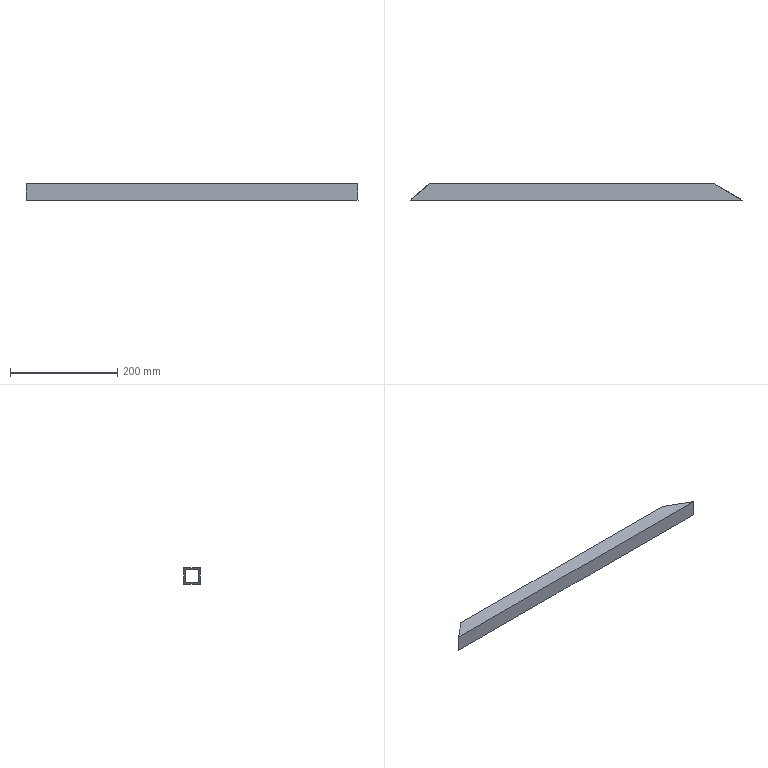Part | NX | features solid 2 | 1 solid | 10 faces | box 620.186 x 30 x 30 mm | volume 129098 mm3 | plane 10
STEP:
#1=CARTESIAN_POINT('',(-71.299,-145.,-75.));
#2=VERTEX_POINT('',#1);
#3=CARTESIAN_POINT('',(461.173,-145.,-75.));
#4=VERTEX_POINT('',#3);
#5=CARTESIAN_POINT('',(25.,-145.,-75.));
#6=DIRECTION('',(1.,0.,0.));
#7=VECTOR('',#6,1000.);
#8=LINE('',#5,#7);
#9=EDGE_CURVE('',#2,#4,#8,.T.);
#10=ORIENTED_EDGE('',*,*,#9,.F.);
#11=CARTESIAN_POINT('',(-71.299,-145.,-45.));
#12=VERTEX_POINT('',#11);
#13=CARTESIAN_POINT('',(-71.299,-145.,-75.));
#14=DIRECTION('',(0.,0.,-1.));
#15=VECTOR('',#14,1000.);
#16=LINE('',#13,#15);
#17=EDGE_CURVE('',#2,#12,#16,.F.);
#18=ORIENTED_EDGE('',*,*,#17,.T.);
#19=CARTESIAN_POINT('',(461.173,-145.,-45.));
#20=VERTEX_POINT('',#19);
#21=CARTESIAN_POINT('',(25.,-145.,-45.));
#22=DIRECTION('',(1.,0.,0.));
#23=VECTOR('',#22,1000.);
#24=LINE('',#21,#23);
#25=EDGE_CURVE('',#12,#20,#24,.T.);
#26=ORIENTED_EDGE('',*,*,#25,.T.);
#27=CARTESIAN_POINT('',(461.173,-145.,-103.));
#28=DIRECTION('',(0.,0.,-1.));
#29=VECTOR('',#28,1000.);
#30=LINE('',#27,#29);
#31=EDGE_CURVE('',#4,#20,#30,.F.);
#32=ORIENTED_EDGE('',*,*,#31,.F.);
#33=EDGE_LOOP('',(#10,#18,#26,#32));
#34=FACE_BOUND('',#33,.T.);
#35=CARTESIAN_POINT('',(25.,-145.,-75.));
#36=DIRECTION('',(0.,-1.,0.));
#37=DIRECTION('',(1.,0.,0.));
#38=AXIS2_PLACEMENT_3D('',#35,#36,#37);
#39=PLANE('',#38);
#40=ADVANCED_FACE('',(#34),#39,.F.);
#41=CARTESIAN_POINT('',(-107.052,-175.,-45.));
#42=VERTEX_POINT('',#41);
#43=CARTESIAN_POINT('',(-107.052,-175.,-75.));
#44=VERTEX_POINT('',#43);
#45=CARTESIAN_POINT('',(-107.052,-175.,-75.));
#46=DIRECTION('',(0.,0.,-1.));
#47=VECTOR('',#46,1000.);
#48=LINE('',#45,#47);
#49=EDGE_CURVE('',#42,#44,#48,.T.);
#50=ORIENTED_EDGE('',*,*,#49,.T.);
#51=CARTESIAN_POINT('',(513.135,-175.,-75.));
#52=VERTEX_POINT('',#51);
#53=CARTESIAN_POINT('',(25.,-175.,-75.));
#54=DIRECTION('',(1.,0.,0.));
#55=VECTOR('',#54,1000.);
#56=LINE('',#53,#55);
#57=EDGE_CURVE('',#44,#52,#56,.T.);
#58=ORIENTED_EDGE('',*,*,#57,.T.);
#59=CARTESIAN_POINT('',(513.135,-175.,-45.));
#60=VERTEX_POINT('',#59);
#61=CARTESIAN_POINT('',(513.135,-175.,-75.));
#62=DIRECTION('',(0.,0.,1.));
#63=VECTOR('',#62,1000.);
#64=LINE('',#61,#63);
#65=EDGE_CURVE('',#52,#60,#64,.T.);
#66=ORIENTED_EDGE('',*,*,#65,.T.);
#67=CARTESIAN_POINT('',(25.,-175.,-45.));
#68=DIRECTION('',(1.,0.,0.));
#69=VECTOR('',#68,1000.);
#70=LINE('',#67,#69);
#71=EDGE_CURVE('',#42,#60,#70,.T.);
#72=ORIENTED_EDGE('',*,*,#71,.F.);
#73=EDGE_LOOP('',(#50,#58,#66,#72));
#74=FACE_BOUND('',#73,.T.);
#75=CARTESIAN_POINT('',(25.,-175.,-75.));
#76=DIRECTION('',(0.,-1.,0.));
#77=DIRECTION('',(1.,0.,0.));
#78=AXIS2_PLACEMENT_3D('',#75,#76,#77);
#79=PLANE('',#78);
#80=ADVANCED_FACE('',(#74),#79,.T.);
#81=CARTESIAN_POINT('',(-73.683,-147.,-73.));
#82=VERTEX_POINT('',#81);
#83=CARTESIAN_POINT('',(-73.683,-147.,-47.));
#84=VERTEX_POINT('',#83);
#85=CARTESIAN_POINT('',(-73.683,-147.,-75.));
#86=DIRECTION('',(0.,0.,-1.));
#87=VECTOR('',#86,1000.);
#88=LINE('',#85,#87);
#89=EDGE_CURVE('',#82,#84,#88,.F.);
#90=ORIENTED_EDGE('',*,*,#89,.F.);
#91=CARTESIAN_POINT('',(464.637,-147.,-73.));
#92=VERTEX_POINT('',#91);
#93=CARTESIAN_POINT('',(25.,-147.,-73.));
#94=DIRECTION('',(-1.,0.,0.));
#95=VECTOR('',#94,1000.);
#96=LINE('',#93,#95);
#97=EDGE_CURVE('',#82,#92,#96,.F.);
#98=ORIENTED_EDGE('',*,*,#97,.T.);
#99=CARTESIAN_POINT('',(464.637,-147.,-47.));
#100=VERTEX_POINT('',#99);
#101=CARTESIAN_POINT('',(464.637,-147.,-103.));
#102=DIRECTION('',(0.,0.,-1.));
#103=VECTOR('',#102,1000.);
#104=LINE('',#101,#103);
#105=EDGE_CURVE('',#92,#100,#104,.F.);
#106=ORIENTED_EDGE('',*,*,#105,.T.);
#107=CARTESIAN_POINT('',(25.,-147.,-47.));
#108=DIRECTION('',(-1.,0.,0.));
#109=VECTOR('',#108,1000.);
#110=LINE('',#107,#109);
#111=EDGE_CURVE('',#84,#100,#110,.F.);
#112=ORIENTED_EDGE('',*,*,#111,.F.);
#113=EDGE_LOOP('',(#90,#98,#106,#112));
#114=FACE_BOUND('',#113,.T.);
#115=CARTESIAN_POINT('',(25.,-147.,-75.));
#116=DIRECTION('',(0.,-1.,0.));
#117=DIRECTION('',(1.,0.,0.));
#118=AXIS2_PLACEMENT_3D('',#115,#116,#117);
#119=PLANE('',#118);
#120=ADVANCED_FACE('',(#114),#119,.T.);
#121=CARTESIAN_POINT('',(-104.668,-173.,-73.));
#122=VERTEX_POINT('',#121);
#123=CARTESIAN_POINT('',(509.671,-173.,-73.));
#124=VERTEX_POINT('',#123);
#125=CARTESIAN_POINT('',(25.,-173.,-73.));
#126=DIRECTION('',(1.,0.,0.));
#127=VECTOR('',#126,1000.);
#128=LINE('',#125,#127);
#129=EDGE_CURVE('',#122,#124,#128,.T.);
#130=ORIENTED_EDGE('',*,*,#129,.F.);
#131=CARTESIAN_POINT('',(-104.668,-173.,-47.));
#132=VERTEX_POINT('',#131);
#133=CARTESIAN_POINT('',(-104.668,-173.,-75.));
#134=DIRECTION('',(0.,0.,-1.));
#135=VECTOR('',#134,1000.);
#136=LINE('',#133,#135);
#137=EDGE_CURVE('',#132,#122,#136,.T.);
#138=ORIENTED_EDGE('',*,*,#137,.F.);
#139=CARTESIAN_POINT('',(509.671,-173.,-47.));
#140=VERTEX_POINT('',#139);
#141=CARTESIAN_POINT('',(25.,-173.,-47.));
#142=DIRECTION('',(1.,0.,0.));
#143=VECTOR('',#142,1000.);
#144=LINE('',#141,#143);
#145=EDGE_CURVE('',#132,#140,#144,.T.);
#146=ORIENTED_EDGE('',*,*,#145,.T.);
#147=CARTESIAN_POINT('',(509.671,-173.,-75.));
#148=DIRECTION('',(0.,0.,1.));
#149=VECTOR('',#148,1000.);
#150=LINE('',#147,#149);
#151=EDGE_CURVE('',#124,#140,#150,.T.);
#152=ORIENTED_EDGE('',*,*,#151,.F.);
#153=EDGE_LOOP('',(#130,#138,#146,#152));
#154=FACE_BOUND('',#153,.T.);
#155=CARTESIAN_POINT('',(25.,-173.,-75.));
#156=DIRECTION('',(0.,-1.,0.));
#157=DIRECTION('',(1.,0.,0.));
#158=AXIS2_PLACEMENT_3D('',#155,#156,#157);
#159=PLANE('',#158);
#160=ADVANCED_FACE('',(#154),#159,.F.);
#161=CARTESIAN_POINT('',(-123.209,-188.558,-75.));
#162=DIRECTION('',(0.766,0.6428,0.));
#163=VECTOR('',#162,1000.);
#164=LINE('',#161,#163);
#165=EDGE_CURVE('',#44,#2,#164,.T.);
#166=ORIENTED_EDGE('',*,*,#165,.F.);
#167=ORIENTED_EDGE('',*,*,#49,.F.);
#168=CARTESIAN_POINT('',(-29.561,-109.977,-45.));
#169=DIRECTION('',(-0.766,-0.6428,0.));
#170=VECTOR('',#169,1000.);
#171=LINE('',#168,#170);
#172=EDGE_CURVE('',#12,#42,#171,.T.);
#173=ORIENTED_EDGE('',*,*,#172,.F.);
#174=ORIENTED_EDGE('',*,*,#17,.F.);
#175=EDGE_LOOP('',(#166,#167,#173,#174));
#176=FACE_BOUND('',#175,.T.);
#177=ORIENTED_EDGE('',*,*,#137,.T.);
#178=CARTESIAN_POINT('',(-123.209,-188.558,-73.));
#179=DIRECTION('',(0.766,0.6428,0.));
#180=VECTOR('',#179,1000.);
#181=LINE('',#178,#180);
#182=EDGE_CURVE('',#122,#82,#181,.T.);
#183=ORIENTED_EDGE('',*,*,#182,.T.);
#184=ORIENTED_EDGE('',*,*,#89,.T.);
#185=CARTESIAN_POINT('',(-29.561,-109.977,-47.));
#186=DIRECTION('',(-0.766,-0.6428,0.));
#187=VECTOR('',#186,1000.);
#188=LINE('',#185,#187);
#189=EDGE_CURVE('',#84,#132,#188,.T.);
#190=ORIENTED_EDGE('',*,*,#189,.T.);
#191=EDGE_LOOP('',(#177,#183,#184,#190));
#192=FACE_BOUND('',#191,.T.);
#193=CARTESIAN_POINT('',(-123.209,-188.558,-105.));
#194=DIRECTION('',(-0.6428,0.766,0.));
#195=DIRECTION('',(0.,0.,1.));
#196=AXIS2_PLACEMENT_3D('',#193,#194,#195);
#197=PLANE('',#196);
#198=ADVANCED_FACE('',(#176,#192),#197,.T.);
#199=ORIENTED_EDGE('',*,*,#25,.F.);
#200=ORIENTED_EDGE('',*,*,#172,.T.);
#201=ORIENTED_EDGE('',*,*,#71,.T.);
#202=CARTESIAN_POINT('',(147.034,36.369,-45.));
#203=DIRECTION('',(-0.866,0.5,0.));
#204=VECTOR('',#203,1000.);
#205=LINE('',#202,#204);
#206=EDGE_CURVE('',#60,#20,#205,.T.);
#207=ORIENTED_EDGE('',*,*,#206,.T.);
#208=EDGE_LOOP('',(#199,#200,#201,#207));
#209=FACE_BOUND('',#208,.T.);
#210=CARTESIAN_POINT('',(25.,-175.,-45.));
#211=DIRECTION('',(0.,0.,1.));
#212=DIRECTION('',(1.,0.,0.));
#213=AXIS2_PLACEMENT_3D('',#210,#211,#212);
#214=PLANE('',#213);
#215=ADVANCED_FACE('',(#209),#214,.T.);
#216=ORIENTED_EDGE('',*,*,#57,.F.);
#217=ORIENTED_EDGE('',*,*,#165,.T.);
#218=ORIENTED_EDGE('',*,*,#9,.T.);
#219=CARTESIAN_POINT('',(147.034,36.369,-75.));
#220=DIRECTION('',(-0.866,0.5,0.));
#221=VECTOR('',#220,1000.);
#222=LINE('',#219,#221);
#223=EDGE_CURVE('',#52,#4,#222,.T.);
#224=ORIENTED_EDGE('',*,*,#223,.F.);
#225=EDGE_LOOP('',(#216,#217,#218,#224));
#226=FACE_BOUND('',#225,.T.);
#227=CARTESIAN_POINT('',(25.,-175.,-75.));
#228=DIRECTION('',(0.,0.,1.));
#229=DIRECTION('',(1.,0.,0.));
#230=AXIS2_PLACEMENT_3D('',#227,#228,#229);
#231=PLANE('',#230);
#232=ADVANCED_FACE('',(#226),#231,.F.);
#233=ORIENTED_EDGE('',*,*,#65,.F.);
#234=ORIENTED_EDGE('',*,*,#223,.T.);
#235=ORIENTED_EDGE('',*,*,#31,.T.);
#236=ORIENTED_EDGE('',*,*,#206,.F.);
#237=EDGE_LOOP('',(#233,#234,#235,#236));
#238=FACE_BOUND('',#237,.T.);
#239=CARTESIAN_POINT('',(147.034,36.369,-73.));
#240=DIRECTION('',(-0.866,0.5,0.));
#241=VECTOR('',#240,1000.);
#242=LINE('',#239,#241);
#243=EDGE_CURVE('',#124,#92,#242,.T.);
#244=ORIENTED_EDGE('',*,*,#243,.F.);
#245=ORIENTED_EDGE('',*,*,#151,.T.);
#246=CARTESIAN_POINT('',(147.034,36.369,-47.));
#247=DIRECTION('',(-0.866,0.5,0.));
#248=VECTOR('',#247,1000.);
#249=LINE('',#246,#248);
#250=EDGE_CURVE('',#140,#100,#249,.T.);
#251=ORIENTED_EDGE('',*,*,#250,.T.);
#252=ORIENTED_EDGE('',*,*,#105,.F.);
#253=EDGE_LOOP('',(#244,#245,#251,#252));
#254=FACE_BOUND('',#253,.T.);
#255=CARTESIAN_POINT('',(476.795,-154.019,-103.));
#256=DIRECTION('',(0.5,0.866,0.));
#257=DIRECTION('',(0.,0.,-1.));
#258=AXIS2_PLACEMENT_3D('',#255,#256,#257);
#259=PLANE('',#258);
#260=ADVANCED_FACE('',(#238,#254),#259,.T.);
#261=ORIENTED_EDGE('',*,*,#189,.F.);
#262=ORIENTED_EDGE('',*,*,#111,.T.);
#263=ORIENTED_EDGE('',*,*,#250,.F.);
#264=ORIENTED_EDGE('',*,*,#145,.F.);
#265=EDGE_LOOP('',(#261,#262,#263,#264));
#266=FACE_BOUND('',#265,.T.);
#267=CARTESIAN_POINT('',(25.,-175.,-47.));
#268=DIRECTION('',(0.,0.,1.));
#269=DIRECTION('',(1.,0.,0.));
#270=AXIS2_PLACEMENT_3D('',#267,#268,#269);
#271=PLANE('',#270);
#272=ADVANCED_FACE('',(#266),#271,.F.);
#273=ORIENTED_EDGE('',*,*,#182,.F.);
#274=ORIENTED_EDGE('',*,*,#129,.T.);
#275=ORIENTED_EDGE('',*,*,#243,.T.);
#276=ORIENTED_EDGE('',*,*,#97,.F.);
#277=EDGE_LOOP('',(#273,#274,#275,#276));
#278=FACE_BOUND('',#277,.T.);
#279=CARTESIAN_POINT('',(25.,-175.,-73.));
#280=DIRECTION('',(0.,0.,1.));
#281=DIRECTION('',(1.,0.,0.));
#282=AXIS2_PLACEMENT_3D('',#279,#280,#281);
#283=PLANE('',#282);
#284=ADVANCED_FACE('',(#278),#283,.T.);
#285=CLOSED_SHELL('',(#40,#80,#120,#160,#198,#215,#232,#260,#272,#284));
#286=MANIFOLD_SOLID_BREP('',#285);
#287=(LENGTH_UNIT()NAMED_UNIT(*)SI_UNIT(.MILLI.,.METRE.));
#288=UNCERTAINTY_MEASURE_WITH_UNIT(LENGTH_MEASURE(0.00001),#287,'','');
#289=(NAMED_UNIT(*)PLANE_ANGLE_UNIT()SI_UNIT($,.RADIAN.));
#290=(NAMED_UNIT(*)SI_UNIT($,.STERADIAN.)SOLID_ANGLE_UNIT());
#291=(GEOMETRIC_REPRESENTATION_CONTEXT(3)GLOBAL_UNCERTAINTY_ASSIGNED_CONTEXT((#288))GLOBAL_UNIT_ASSIGNED_CONTEXT((#287,#289,#290))REPRESENTATION_CONTEXT('',''));
#292=ADVANCED_BREP_SHAPE_REPRESENTATION('',(#286),#291);